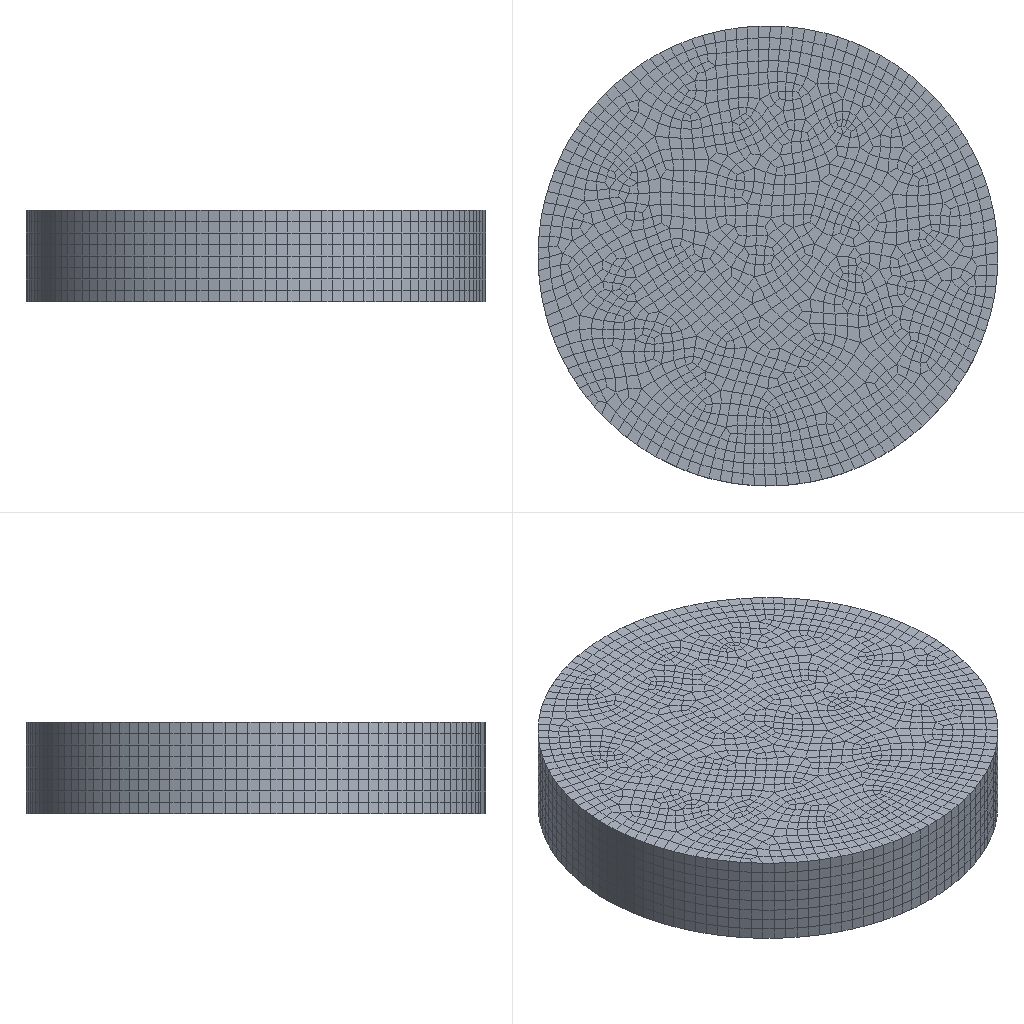Simulation study | abaqus
Set-up summary:
category,name,step,type,value,unit,region
solver,abaqus
solver,version,,,Abaqus/Standard 2020
units,not stated in the deck,,not stated
analysis,deck,,transient,transient
load_step,Step-1,Step-1,transient,nlgeom=True
contact,interactions,,,general=0 pairs=0 ties=0
load_step,requested,,,1
mesh,nodes,,,14931
mesh,elements,,,12760
element_type,C3D8R,,solid,12760
load,load commands in deck,,count,1
bc,support commands in deck,,count,1
material,MATERIAL-1,,in results
check,setup vs results,,match,"per instance, exact: element labels, types and connectivity; labels of the nodes the elements use; coordinates of those nodes at SINGLE_PRECISION in 1 of 1 instance(s)"
Abaqus input file, long lists of numbers shortened:
*Heading
** Job name: Job-1 Model name: Model-1
** Generated by: Abaqus/CAE 2020
*Preprint, echo=NO, model=NO, history=NO, contact=NO
**
** PARTS
**
*Part, name=Part-1
*Node
      1,   20.175,  -22.202,           0.
      2,   23.259,  -18.948,           0.
** (14929 more lines like these left out)
*Element, type=C3D8R
    1,  2011,  1705,  2320,  1685,   352,    46,   661,    26
    2,  1849,  2134,  2320,  2235,   190,   475,   661,   576
** (12758 more lines like these left out)
*Nset, nset=Set-1, generate
     1,  14931,      1
*Elset, elset=Set-1, generate
     1,  12760,      1
** Section: Section-1
*Solid Section, elset=Set-1, material=Material-1
,
*End Part
**
**
** ASSEMBLY
**
*Assembly, name=Assembly
**
*Instance, name=Part-1-1, part=Part-1
*End Instance
**
*Nset, nset=Set-1, instance=Part-1-1, generate
    1,  1659,     1
*Elset, elset=Set-1, instance=Part-1-1, generate
    1,  1595,     1
*End Assembly
**
** MATERIALS
**
*Material, name=Material-1
*Density
 1.2e-09,
*Elastic
3000., 0.38
** ----------------------------------------------------------------
**
** STEP: Step-1
**
*Step, name=Step-1, nlgeom=YES, inc=1000
*Dynamic
0.001,0.02,1e-07
**
** BOUNDARY CONDITIONS
**
** Name: BC-1 Type: 位移/转角
*Boundary
Set-1, 3, 3
**
** LOADS
**
** Name: Load-1   Type: Gravity
*Dload
, GRAV, 1.96e+08, 0., 0., -1.
**
** OUTPUT REQUESTS
**
*Restart, write, frequency=0
**
** FIELD OUTPUT: F-Output-1
**
*Output, field
*Node Output
A, CF, RF, RM, RT, TF, U, V
*Element Output, directions=YES
E, LE, MISES, MISESMAX, MISESONLY, PE, PEEQ, PEEQMAX, PEEQT, PEMAG, S, SF, SSAVG, YIELDPOT
*Contact Output
CDISP, CSTRESS
**
** HISTORY OUTPUT: H-Output-1
**
*Output, history, variable=PRESELECT
*End Step
Results summary:
result,step,,completed,increments=77 time=0.02/0.02
result,analysis,,,transient
result,last_loadstep,,,1
result,analysis steps,,count,1
result,primary field,,,U
result,reaction total,,FX,0.0,model units
result,reaction total,,FY,0.0,model units
result,reaction total,,FZ,7979.87,model units